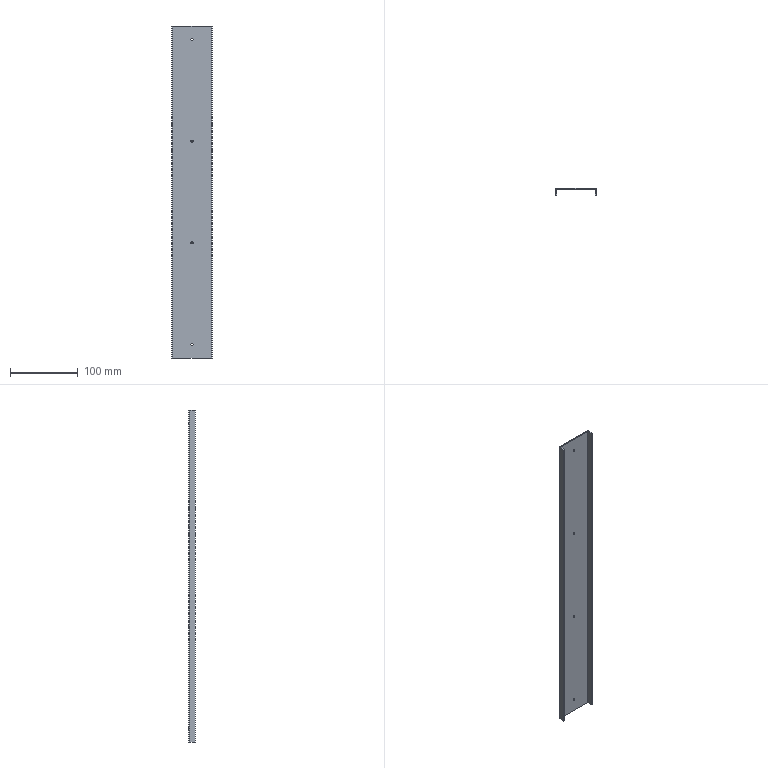Part | STEP file | 1 solid | 30 faces | box 60 x 10 x 490 mm | volume 55944 mm3 | plane 18 | cylinder 12 | commonest cylinder face diameters 3.3 x8 0.4 x2 3.4 x2